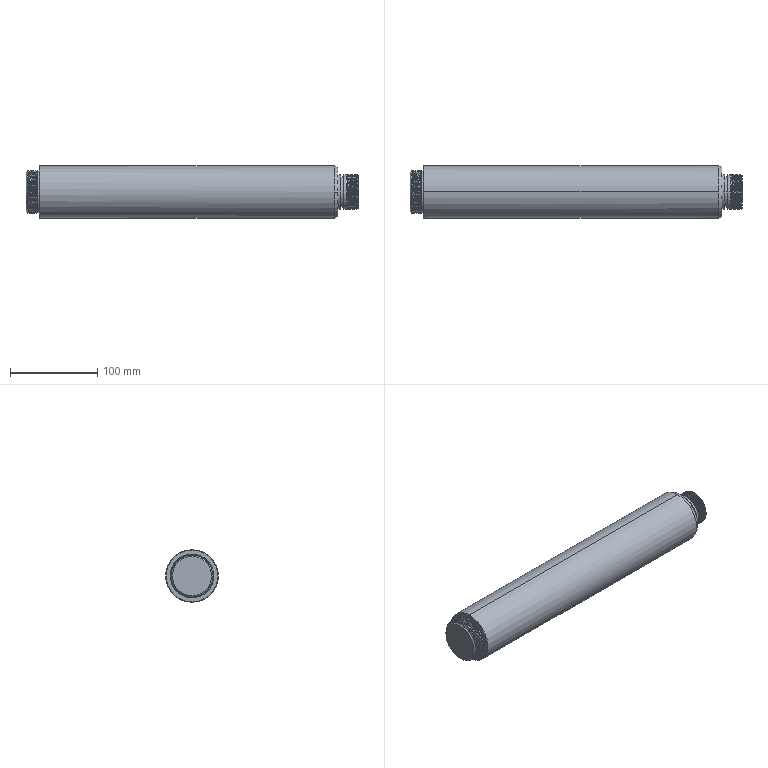Part | SolidWorks | features BaseBody 1 | 1 solid | 98 faces | box 379.7 x 60 x 60 mm | volume 998065 mm3 | cylinder 63 | plane 13 | cone 12 | spline 10 | commonest cylinder face diameters 25 x22 39 x17 50 x12 40 x4 30 x2 35.4 x2